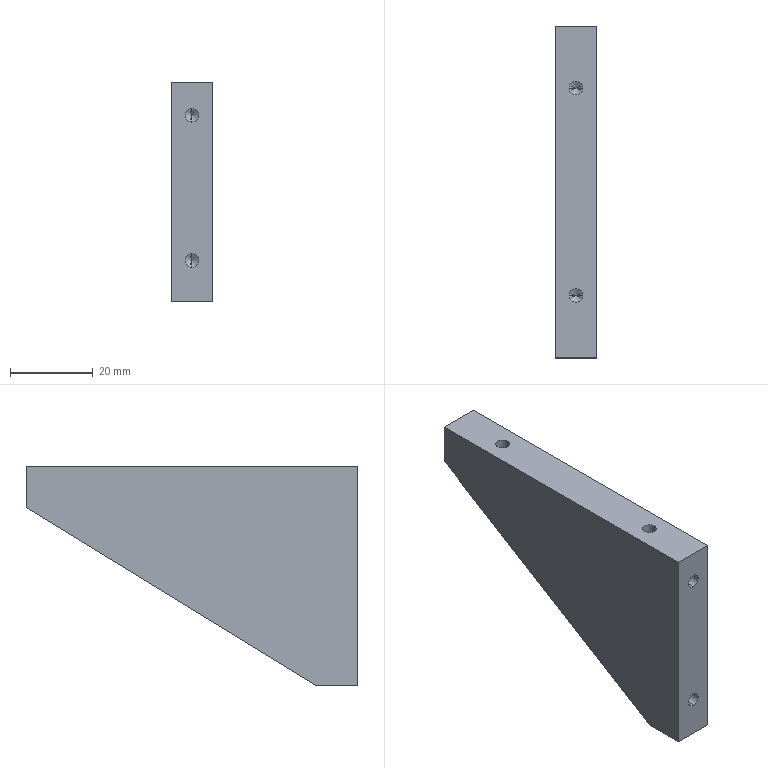Part | SolidWorks | features HoleWzd 2, Extrusion 1 | 1 solid | 23 faces | box 10 x 80 x 53 mm | volume 26993 mm3 | cylinder 8 | cone 8 | plane 7 | commonest cylinder face diameters 3.3 x8
STEP:
#1=CARTESIAN_POINT('',(5.,10.1,-41.35));
#2=VERTEX_POINT('',#1);
#3=CARTESIAN_POINT('',(5.,10.1,-44.65));
#4=VERTEX_POINT('',#3);
#5=CARTESIAN_POINT('',(5.,10.1,-43.));
#6=DIRECTION('',(0.,-1.,0.));
#7=DIRECTION('',(0.,0.,-1.));
#8=AXIS2_PLACEMENT_3D('',#5,#6,#7);
#9=CIRCLE('',#8,1.65);
#10=EDGE_CURVE('',#2,#4,#9,.T.);
#11=ORIENTED_EDGE('',*,*,#10,.F.);
#12=CARTESIAN_POINT('',(5.,0.,-41.35));
#13=VERTEX_POINT('',#12);
#14=CARTESIAN_POINT('',(5.,0.,-41.35));
#15=DIRECTION('',(0.,-1.,0.));
#16=VECTOR('',#15,1000.);
#17=LINE('',#14,#16);
#18=EDGE_CURVE('',#2,#13,#17,.T.);
#19=ORIENTED_EDGE('',*,*,#18,.T.);
#20=CARTESIAN_POINT('',(5.,0.,-44.65));
#21=VERTEX_POINT('',#20);
#22=CARTESIAN_POINT('',(5.,0.,-43.));
#23=DIRECTION('',(0.,-1.,0.));
#24=DIRECTION('',(0.,0.,-1.));
#25=AXIS2_PLACEMENT_3D('',#22,#23,#24);
#26=CIRCLE('',#25,1.65);
#27=EDGE_CURVE('',#13,#21,#26,.T.);
#28=ORIENTED_EDGE('',*,*,#27,.T.);
#29=CARTESIAN_POINT('',(5.,0.,-44.65));
#30=DIRECTION('',(0.,-1.,0.));
#31=VECTOR('',#30,1000.);
#32=LINE('',#29,#31);
#33=EDGE_CURVE('',#4,#21,#32,.T.);
#34=ORIENTED_EDGE('',*,*,#33,.F.);
#35=EDGE_LOOP('',(#11,#19,#28,#34));
#36=FACE_OUTER_BOUND('',#35,.T.);
#37=CARTESIAN_POINT('',(5.,0.,-43.));
#38=DIRECTION('',(0.,-1.,0.));
#39=DIRECTION('',(0.,0.,-1.));
#40=AXIS2_PLACEMENT_3D('',#37,#38,#39);
#41=CYLINDRICAL_SURFACE('',#40,1.65);
#42=ADVANCED_FACE('',(#36),#41,.F.);
#43=CARTESIAN_POINT('',(5.,11.091,-43.));
#44=VERTEX_POINT('',#43);
#45=CARTESIAN_POINT('',(5.,10.1,-44.65));
#46=DIRECTION('',(0.,-0.515,-0.8572));
#47=VECTOR('',#46,1000.);
#48=LINE('',#45,#47);
#49=EDGE_CURVE('',#44,#4,#48,.T.);
#50=ORIENTED_EDGE('',*,*,#49,.F.);
#51=CARTESIAN_POINT('',(5.,10.1,-41.35));
#52=DIRECTION('',(0.,-0.515,0.8572));
#53=VECTOR('',#52,1000.);
#54=LINE('',#51,#53);
#55=EDGE_CURVE('',#44,#2,#54,.T.);
#56=ORIENTED_EDGE('',*,*,#55,.T.);
#57=ORIENTED_EDGE('',*,*,#10,.T.);
#58=EDGE_LOOP('',(#50,#56,#57));
#59=FACE_OUTER_BOUND('',#58,.T.);
#60=CARTESIAN_POINT('',(5.,10.1,-43.));
#61=DIRECTION('',(0.,-1.,0.));
#62=DIRECTION('',(0.,0.,-1.));
#63=AXIS2_PLACEMENT_3D('',#60,#61,#62);
#64=CONICAL_SURFACE('',#63,1.65,1.03);
#65=ADVANCED_FACE('',(#59),#64,.F.);
#66=CARTESIAN_POINT('',(5.,10.1,-6.35));
#67=VERTEX_POINT('',#66);
#68=CARTESIAN_POINT('',(5.,10.1,-9.65));
#69=VERTEX_POINT('',#68);
#70=CARTESIAN_POINT('',(5.,10.1,-8.));
#71=DIRECTION('',(0.,-1.,0.));
#72=DIRECTION('',(0.,0.,-1.));
#73=AXIS2_PLACEMENT_3D('',#70,#71,#72);
#74=CIRCLE('',#73,1.65);
#75=EDGE_CURVE('',#67,#69,#74,.T.);
#76=ORIENTED_EDGE('',*,*,#75,.F.);
#77=CARTESIAN_POINT('',(5.,0.,-6.35));
#78=VERTEX_POINT('',#77);
#79=CARTESIAN_POINT('',(5.,0.,-6.35));
#80=DIRECTION('',(0.,-1.,0.));
#81=VECTOR('',#80,1000.);
#82=LINE('',#79,#81);
#83=EDGE_CURVE('',#67,#78,#82,.T.);
#84=ORIENTED_EDGE('',*,*,#83,.T.);
#85=CARTESIAN_POINT('',(5.,0.,-9.65));
#86=VERTEX_POINT('',#85);
#87=CARTESIAN_POINT('',(5.,0.,-8.));
#88=DIRECTION('',(0.,-1.,0.));
#89=DIRECTION('',(0.,0.,-1.));
#90=AXIS2_PLACEMENT_3D('',#87,#88,#89);
#91=CIRCLE('',#90,1.65);
#92=EDGE_CURVE('',#78,#86,#91,.T.);
#93=ORIENTED_EDGE('',*,*,#92,.T.);
#94=CARTESIAN_POINT('',(5.,0.,-9.65));
#95=DIRECTION('',(0.,-1.,0.));
#96=VECTOR('',#95,1000.);
#97=LINE('',#94,#96);
#98=EDGE_CURVE('',#69,#86,#97,.T.);
#99=ORIENTED_EDGE('',*,*,#98,.F.);
#100=EDGE_LOOP('',(#76,#84,#93,#99));
#101=FACE_OUTER_BOUND('',#100,.T.);
#102=CARTESIAN_POINT('',(5.,0.,-8.));
#103=DIRECTION('',(0.,-1.,0.));
#104=DIRECTION('',(0.,0.,-1.));
#105=AXIS2_PLACEMENT_3D('',#102,#103,#104);
#106=CYLINDRICAL_SURFACE('',#105,1.65);
#107=ADVANCED_FACE('',(#101),#106,.F.);
#108=CARTESIAN_POINT('',(5.,11.091,-8.));
#109=VERTEX_POINT('',#108);
#110=CARTESIAN_POINT('',(5.,10.1,-9.65));
#111=DIRECTION('',(0.,-0.515,-0.8572));
#112=VECTOR('',#111,1000.);
#113=LINE('',#110,#112);
#114=EDGE_CURVE('',#109,#69,#113,.T.);
#115=ORIENTED_EDGE('',*,*,#114,.F.);
#116=CARTESIAN_POINT('',(5.,10.1,-6.35));
#117=DIRECTION('',(0.,-0.515,0.8572));
#118=VECTOR('',#117,1000.);
#119=LINE('',#116,#118);
#120=EDGE_CURVE('',#109,#67,#119,.T.);
#121=ORIENTED_EDGE('',*,*,#120,.T.);
#122=ORIENTED_EDGE('',*,*,#75,.T.);
#123=EDGE_LOOP('',(#115,#121,#122));
#124=FACE_OUTER_BOUND('',#123,.T.);
#125=CARTESIAN_POINT('',(5.,10.1,-8.));
#126=DIRECTION('',(0.,-1.,0.));
#127=DIRECTION('',(0.,0.,-1.));
#128=AXIS2_PLACEMENT_3D('',#125,#126,#127);
#129=CONICAL_SURFACE('',#128,1.65,1.03);
#130=ADVANCED_FACE('',(#124),#129,.F.);
#131=CARTESIAN_POINT('',(3.35,65.,-10.1));
#132=VERTEX_POINT('',#131);
#133=CARTESIAN_POINT('',(6.65,65.,-10.1));
#134=VERTEX_POINT('',#133);
#135=CARTESIAN_POINT('',(5.,65.,-10.1));
#136=DIRECTION('',(0.,0.,1.));
#137=DIRECTION('',(1.,0.,0.));
#138=AXIS2_PLACEMENT_3D('',#135,#136,#137);
#139=CIRCLE('',#138,1.65);
#140=EDGE_CURVE('',#132,#134,#139,.T.);
#141=ORIENTED_EDGE('',*,*,#140,.F.);
#142=CARTESIAN_POINT('',(3.35,65.,0.));
#143=VERTEX_POINT('',#142);
#144=CARTESIAN_POINT('',(3.35,65.,0.));
#145=DIRECTION('',(0.,0.,1.));
#146=VECTOR('',#145,1000.);
#147=LINE('',#144,#146);
#148=EDGE_CURVE('',#132,#143,#147,.T.);
#149=ORIENTED_EDGE('',*,*,#148,.T.);
#150=CARTESIAN_POINT('',(6.65,65.,0.));
#151=VERTEX_POINT('',#150);
#152=CARTESIAN_POINT('',(5.,65.,0.));
#153=DIRECTION('',(0.,0.,1.));
#154=DIRECTION('',(1.,0.,0.));
#155=AXIS2_PLACEMENT_3D('',#152,#153,#154);
#156=CIRCLE('',#155,1.65);
#157=EDGE_CURVE('',#143,#151,#156,.T.);
#158=ORIENTED_EDGE('',*,*,#157,.T.);
#159=CARTESIAN_POINT('',(6.65,65.,0.));
#160=DIRECTION('',(0.,0.,1.));
#161=VECTOR('',#160,1000.);
#162=LINE('',#159,#161);
#163=EDGE_CURVE('',#134,#151,#162,.T.);
#164=ORIENTED_EDGE('',*,*,#163,.F.);
#165=EDGE_LOOP('',(#141,#149,#158,#164));
#166=FACE_OUTER_BOUND('',#165,.T.);
#167=CARTESIAN_POINT('',(5.,65.,0.));
#168=DIRECTION('',(0.,0.,1.));
#169=DIRECTION('',(1.,0.,0.));
#170=AXIS2_PLACEMENT_3D('',#167,#168,#169);
#171=CYLINDRICAL_SURFACE('',#170,1.65);
#172=ADVANCED_FACE('',(#166),#171,.F.);
#173=CARTESIAN_POINT('',(5.,65.,-11.091));
#174=VERTEX_POINT('',#173);
#175=CARTESIAN_POINT('',(6.65,65.,-10.1));
#176=DIRECTION('',(0.8572,0.,0.515));
#177=VECTOR('',#176,1000.);
#178=LINE('',#175,#177);
#179=EDGE_CURVE('',#174,#134,#178,.T.);
#180=ORIENTED_EDGE('',*,*,#179,.F.);
#181=CARTESIAN_POINT('',(3.35,65.,-10.1));
#182=DIRECTION('',(-0.8572,0.,0.515));
#183=VECTOR('',#182,1000.);
#184=LINE('',#181,#183);
#185=EDGE_CURVE('',#174,#132,#184,.T.);
#186=ORIENTED_EDGE('',*,*,#185,.T.);
#187=ORIENTED_EDGE('',*,*,#140,.T.);
#188=EDGE_LOOP('',(#180,#186,#187));
#189=FACE_OUTER_BOUND('',#188,.T.);
#190=CARTESIAN_POINT('',(5.,65.,-10.1));
#191=DIRECTION('',(0.,0.,1.));
#192=DIRECTION('',(1.,0.,0.));
#193=AXIS2_PLACEMENT_3D('',#190,#191,#192);
#194=CONICAL_SURFACE('',#193,1.65,1.03);
#195=ADVANCED_FACE('',(#189),#194,.F.);
#196=CARTESIAN_POINT('',(3.35,15.,-10.1));
#197=VERTEX_POINT('',#196);
#198=CARTESIAN_POINT('',(6.65,15.,-10.1));
#199=VERTEX_POINT('',#198);
#200=CARTESIAN_POINT('',(5.,15.,-10.1));
#201=DIRECTION('',(0.,0.,1.));
#202=DIRECTION('',(1.,0.,0.));
#203=AXIS2_PLACEMENT_3D('',#200,#201,#202);
#204=CIRCLE('',#203,1.65);
#205=EDGE_CURVE('',#197,#199,#204,.T.);
#206=ORIENTED_EDGE('',*,*,#205,.F.);
#207=CARTESIAN_POINT('',(3.35,15.,0.));
#208=VERTEX_POINT('',#207);
#209=CARTESIAN_POINT('',(3.35,15.,0.));
#210=DIRECTION('',(0.,0.,1.));
#211=VECTOR('',#210,1000.);
#212=LINE('',#209,#211);
#213=EDGE_CURVE('',#197,#208,#212,.T.);
#214=ORIENTED_EDGE('',*,*,#213,.T.);
#215=CARTESIAN_POINT('',(6.65,15.,0.));
#216=VERTEX_POINT('',#215);
#217=CARTESIAN_POINT('',(5.,15.,0.));
#218=DIRECTION('',(0.,0.,1.));
#219=DIRECTION('',(1.,0.,0.));
#220=AXIS2_PLACEMENT_3D('',#217,#218,#219);
#221=CIRCLE('',#220,1.65);
#222=EDGE_CURVE('',#208,#216,#221,.T.);
#223=ORIENTED_EDGE('',*,*,#222,.T.);
#224=CARTESIAN_POINT('',(6.65,15.,0.));
#225=DIRECTION('',(0.,0.,1.));
#226=VECTOR('',#225,1000.);
#227=LINE('',#224,#226);
#228=EDGE_CURVE('',#199,#216,#227,.T.);
#229=ORIENTED_EDGE('',*,*,#228,.F.);
#230=EDGE_LOOP('',(#206,#214,#223,#229));
#231=FACE_OUTER_BOUND('',#230,.T.);
#232=CARTESIAN_POINT('',(5.,15.,0.));
#233=DIRECTION('',(0.,0.,1.));
#234=DIRECTION('',(1.,0.,0.));
#235=AXIS2_PLACEMENT_3D('',#232,#233,#234);
#236=CYLINDRICAL_SURFACE('',#235,1.65);
#237=ADVANCED_FACE('',(#231),#236,.F.);
#238=CARTESIAN_POINT('',(5.,15.,-11.091));
#239=VERTEX_POINT('',#238);
#240=CARTESIAN_POINT('',(6.65,15.,-10.1));
#241=DIRECTION('',(0.8572,0.,0.515));
#242=VECTOR('',#241,1000.);
#243=LINE('',#240,#242);
#244=EDGE_CURVE('',#239,#199,#243,.T.);
#245=ORIENTED_EDGE('',*,*,#244,.F.);
#246=CARTESIAN_POINT('',(3.35,15.,-10.1));
#247=DIRECTION('',(-0.8572,0.,0.515));
#248=VECTOR('',#247,1000.);
#249=LINE('',#246,#248);
#250=EDGE_CURVE('',#239,#197,#249,.T.);
#251=ORIENTED_EDGE('',*,*,#250,.T.);
#252=ORIENTED_EDGE('',*,*,#205,.T.);
#253=EDGE_LOOP('',(#245,#251,#252));
#254=FACE_OUTER_BOUND('',#253,.T.);
#255=CARTESIAN_POINT('',(5.,15.,-10.1));
#256=DIRECTION('',(0.,0.,1.));
#257=DIRECTION('',(1.,0.,0.));
#258=AXIS2_PLACEMENT_3D('',#255,#256,#257);
#259=CONICAL_SURFACE('',#258,1.65,1.03);
#260=ADVANCED_FACE('',(#254),#259,.F.);
#261=CARTESIAN_POINT('',(5.,0.,-43.));
#262=DIRECTION('',(0.,-1.,0.));
#263=DIRECTION('',(0.,0.,-1.));
#264=AXIS2_PLACEMENT_3D('',#261,#262,#263);
#265=CIRCLE('',#264,1.65);
#266=EDGE_CURVE('',#21,#13,#265,.T.);
#267=ORIENTED_EDGE('',*,*,#266,.F.);
#268=ORIENTED_EDGE('',*,*,#27,.F.);
#269=EDGE_LOOP('',(#267,#268));
#270=FACE_BOUND('',#269,.T.);
#271=CARTESIAN_POINT('',(5.,0.,-8.));
#272=DIRECTION('',(0.,-1.,0.));
#273=DIRECTION('',(0.,0.,-1.));
#274=AXIS2_PLACEMENT_3D('',#271,#272,#273);
#275=CIRCLE('',#274,1.65);
#276=EDGE_CURVE('',#86,#78,#275,.T.);
#277=ORIENTED_EDGE('',*,*,#276,.F.);
#278=ORIENTED_EDGE('',*,*,#92,.F.);
#279=EDGE_LOOP('',(#277,#278));
#280=FACE_BOUND('',#279,.T.);
#281=CARTESIAN_POINT('',(0.,0.,0.));
#282=VERTEX_POINT('',#281);
#283=CARTESIAN_POINT('',(0.,0.,-53.));
#284=VERTEX_POINT('',#283);
#285=CARTESIAN_POINT('',(0.,0.,-53.));
#286=DIRECTION('',(0.,0.,-1.));
#287=VECTOR('',#286,1000.);
#288=LINE('',#285,#287);
#289=EDGE_CURVE('',#282,#284,#288,.T.);
#290=ORIENTED_EDGE('',*,*,#289,.T.);
#291=CARTESIAN_POINT('',(10.,0.,-53.));
#292=VERTEX_POINT('',#291);
#293=CARTESIAN_POINT('',(10.,0.,-53.));
#294=DIRECTION('',(-1.,0.,0.));
#295=VECTOR('',#294,1000.);
#296=LINE('',#293,#295);
#297=EDGE_CURVE('',#292,#284,#296,.T.);
#298=ORIENTED_EDGE('',*,*,#297,.F.);
#299=CARTESIAN_POINT('',(10.,0.,0.));
#300=VERTEX_POINT('',#299);
#301=CARTESIAN_POINT('',(10.,0.,-53.));
#302=DIRECTION('',(0.,0.,-1.));
#303=VECTOR('',#302,1000.);
#304=LINE('',#301,#303);
#305=EDGE_CURVE('',#300,#292,#304,.T.);
#306=ORIENTED_EDGE('',*,*,#305,.F.);
#307=CARTESIAN_POINT('',(10.,0.,0.));
#308=DIRECTION('',(-1.,0.,0.));
#309=VECTOR('',#308,1000.);
#310=LINE('',#307,#309);
#311=EDGE_CURVE('',#300,#282,#310,.T.);
#312=ORIENTED_EDGE('',*,*,#311,.T.);
#313=EDGE_LOOP('',(#290,#298,#306,#312));
#314=FACE_OUTER_BOUND('',#313,.T.);
#315=CARTESIAN_POINT('',(10.,0.,-53.));
#316=DIRECTION('',(0.,1.,0.));
#317=DIRECTION('',(0.,0.,1.));
#318=AXIS2_PLACEMENT_3D('',#315,#316,#317);
#319=PLANE('',#318);
#320=ADVANCED_FACE('',(#270,#280,#314),#319,.F.);
#321=CARTESIAN_POINT('',(0.,10.,-53.));
#322=VERTEX_POINT('',#321);
#323=CARTESIAN_POINT('',(0.,10.,-53.));
#324=DIRECTION('',(0.,1.,0.));
#325=VECTOR('',#324,1000.);
#326=LINE('',#323,#325);
#327=EDGE_CURVE('',#284,#322,#326,.T.);
#328=ORIENTED_EDGE('',*,*,#327,.T.);
#329=CARTESIAN_POINT('',(10.,10.,-53.));
#330=VERTEX_POINT('',#329);
#331=CARTESIAN_POINT('',(10.,10.,-53.));
#332=DIRECTION('',(-1.,0.,0.));
#333=VECTOR('',#332,1000.);
#334=LINE('',#331,#333);
#335=EDGE_CURVE('',#330,#322,#334,.T.);
#336=ORIENTED_EDGE('',*,*,#335,.F.);
#337=CARTESIAN_POINT('',(10.,10.,-53.));
#338=DIRECTION('',(0.,1.,0.));
#339=VECTOR('',#338,1000.);
#340=LINE('',#337,#339);
#341=EDGE_CURVE('',#292,#330,#340,.T.);
#342=ORIENTED_EDGE('',*,*,#341,.F.);
#343=ORIENTED_EDGE('',*,*,#297,.T.);
#344=EDGE_LOOP('',(#328,#336,#342,#343));
#345=FACE_OUTER_BOUND('',#344,.T.);
#346=CARTESIAN_POINT('',(10.,10.,-53.));
#347=DIRECTION('',(0.,0.,1.));
#348=DIRECTION('',(1.,0.,0.));
#349=AXIS2_PLACEMENT_3D('',#346,#347,#348);
#350=PLANE('',#349);
#351=ADVANCED_FACE('',(#345),#350,.F.);
#352=CARTESIAN_POINT('',(0.,80.,-10.));
#353=VERTEX_POINT('',#352);
#354=CARTESIAN_POINT('',(0.,80.,-10.));
#355=DIRECTION('',(0.,0.8521,0.5234));
#356=VECTOR('',#355,1000.);
#357=LINE('',#354,#356);
#358=EDGE_CURVE('',#322,#353,#357,.T.);
#359=ORIENTED_EDGE('',*,*,#358,.T.);
#360=CARTESIAN_POINT('',(10.,80.,-10.));
#361=VERTEX_POINT('',#360);
#362=CARTESIAN_POINT('',(10.,80.,-10.));
#363=DIRECTION('',(-1.,0.,0.));
#364=VECTOR('',#363,1000.);
#365=LINE('',#362,#364);
#366=EDGE_CURVE('',#361,#353,#365,.T.);
#367=ORIENTED_EDGE('',*,*,#366,.F.);
#368=CARTESIAN_POINT('',(10.,80.,-10.));
#369=DIRECTION('',(0.,0.8521,0.5234));
#370=VECTOR('',#369,1000.);
#371=LINE('',#368,#370);
#372=EDGE_CURVE('',#330,#361,#371,.T.);
#373=ORIENTED_EDGE('',*,*,#372,.F.);
#374=ORIENTED_EDGE('',*,*,#335,.T.);
#375=EDGE_LOOP('',(#359,#367,#373,#374));
#376=FACE_OUTER_BOUND('',#375,.T.);
#377=CARTESIAN_POINT('',(10.,80.,-10.));
#378=DIRECTION('',(0.,-0.5234,0.8521));
#379=DIRECTION('',(0.,-0.8521,-0.5234));
#380=AXIS2_PLACEMENT_3D('',#377,#378,#379);
#381=PLANE('',#380);
#382=ADVANCED_FACE('',(#376),#381,.F.);
#383=CARTESIAN_POINT('',(0.,80.,0.));
#384=VERTEX_POINT('',#383);
#385=CARTESIAN_POINT('',(0.,80.,0.));
#386=DIRECTION('',(0.,0.,1.));
#387=VECTOR('',#386,1000.);
#388=LINE('',#385,#387);
#389=EDGE_CURVE('',#353,#384,#388,.T.);
#390=ORIENTED_EDGE('',*,*,#389,.T.);
#391=CARTESIAN_POINT('',(10.,80.,0.));
#392=VERTEX_POINT('',#391);
#393=CARTESIAN_POINT('',(10.,80.,0.));
#394=DIRECTION('',(-1.,0.,0.));
#395=VECTOR('',#394,1000.);
#396=LINE('',#393,#395);
#397=EDGE_CURVE('',#392,#384,#396,.T.);
#398=ORIENTED_EDGE('',*,*,#397,.F.);
#399=CARTESIAN_POINT('',(10.,80.,0.));
#400=DIRECTION('',(0.,0.,1.));
#401=VECTOR('',#400,1000.);
#402=LINE('',#399,#401);
#403=EDGE_CURVE('',#361,#392,#402,.T.);
#404=ORIENTED_EDGE('',*,*,#403,.F.);
#405=ORIENTED_EDGE('',*,*,#366,.T.);
#406=EDGE_LOOP('',(#390,#398,#404,#405));
#407=FACE_OUTER_BOUND('',#406,.T.);
#408=CARTESIAN_POINT('',(10.,80.,0.));
#409=DIRECTION('',(0.,-1.,0.));
#410=DIRECTION('',(0.,0.,-1.));
#411=AXIS2_PLACEMENT_3D('',#408,#409,#410);
#412=PLANE('',#411);
#413=ADVANCED_FACE('',(#407),#412,.F.);
#414=CARTESIAN_POINT('',(5.,65.,0.));
#415=DIRECTION('',(0.,0.,1.));
#416=DIRECTION('',(1.,0.,0.));
#417=AXIS2_PLACEMENT_3D('',#414,#415,#416);
#418=CIRCLE('',#417,1.65);
#419=EDGE_CURVE('',#151,#143,#418,.T.);
#420=ORIENTED_EDGE('',*,*,#419,.F.);
#421=ORIENTED_EDGE('',*,*,#157,.F.);
#422=EDGE_LOOP('',(#420,#421));
#423=FACE_BOUND('',#422,.T.);
#424=CARTESIAN_POINT('',(5.,15.,0.));
#425=DIRECTION('',(0.,0.,1.));
#426=DIRECTION('',(1.,0.,0.));
#427=AXIS2_PLACEMENT_3D('',#424,#425,#426);
#428=CIRCLE('',#427,1.65);
#429=EDGE_CURVE('',#216,#208,#428,.T.);
#430=ORIENTED_EDGE('',*,*,#429,.F.);
#431=ORIENTED_EDGE('',*,*,#222,.F.);
#432=EDGE_LOOP('',(#430,#431));
#433=FACE_BOUND('',#432,.T.);
#434=CARTESIAN_POINT('',(0.,0.,0.));
#435=DIRECTION('',(0.,-1.,0.));
#436=VECTOR('',#435,1000.);
#437=LINE('',#434,#436);
#438=EDGE_CURVE('',#384,#282,#437,.T.);
#439=ORIENTED_EDGE('',*,*,#438,.T.);
#440=ORIENTED_EDGE('',*,*,#311,.F.);
#441=CARTESIAN_POINT('',(10.,0.,0.));
#442=DIRECTION('',(0.,-1.,0.));
#443=VECTOR('',#442,1000.);
#444=LINE('',#441,#443);
#445=EDGE_CURVE('',#392,#300,#444,.T.);
#446=ORIENTED_EDGE('',*,*,#445,.F.);
#447=ORIENTED_EDGE('',*,*,#397,.T.);
#448=EDGE_LOOP('',(#439,#440,#446,#447));
#449=FACE_OUTER_BOUND('',#448,.T.);
#450=CARTESIAN_POINT('',(10.,0.,0.));
#451=DIRECTION('',(0.,0.,-1.));
#452=DIRECTION('',(-1.,0.,0.));
#453=AXIS2_PLACEMENT_3D('',#450,#451,#452);
#454=PLANE('',#453);
#455=ADVANCED_FACE('',(#423,#433,#449),#454,.F.);
#456=ORIENTED_EDGE('',*,*,#305,.T.);
#457=ORIENTED_EDGE('',*,*,#341,.T.);
#458=ORIENTED_EDGE('',*,*,#372,.T.);
#459=ORIENTED_EDGE('',*,*,#403,.T.);
#460=ORIENTED_EDGE('',*,*,#445,.T.);
#461=EDGE_LOOP('',(#456,#457,#458,#459,#460));
#462=FACE_OUTER_BOUND('',#461,.T.);
#463=CARTESIAN_POINT('',(10.,0.,0.));
#464=DIRECTION('',(-1.,0.,0.));
#465=DIRECTION('',(0.,0.,1.));
#466=AXIS2_PLACEMENT_3D('',#463,#464,#465);
#467=PLANE('',#466);
#468=ADVANCED_FACE('',(#462),#467,.F.);
#469=ORIENTED_EDGE('',*,*,#289,.F.);
#470=ORIENTED_EDGE('',*,*,#438,.F.);
#471=ORIENTED_EDGE('',*,*,#389,.F.);
#472=ORIENTED_EDGE('',*,*,#358,.F.);
#473=ORIENTED_EDGE('',*,*,#327,.F.);
#474=EDGE_LOOP('',(#469,#470,#471,#472,#473));
#475=FACE_OUTER_BOUND('',#474,.T.);
#476=CARTESIAN_POINT('',(0.,0.,0.));
#477=DIRECTION('',(-1.,0.,0.));
#478=DIRECTION('',(0.,0.,1.));
#479=AXIS2_PLACEMENT_3D('',#476,#477,#478);
#480=PLANE('',#479);
#481=ADVANCED_FACE('',(#475),#480,.T.);
#482=ORIENTED_EDGE('',*,*,#250,.F.);
#483=ORIENTED_EDGE('',*,*,#244,.T.);
#484=CARTESIAN_POINT('',(5.,15.,-10.1));
#485=DIRECTION('',(0.,0.,1.));
#486=DIRECTION('',(1.,0.,0.));
#487=AXIS2_PLACEMENT_3D('',#484,#485,#486);
#488=CIRCLE('',#487,1.65);
#489=EDGE_CURVE('',#199,#197,#488,.T.);
#490=ORIENTED_EDGE('',*,*,#489,.T.);
#491=EDGE_LOOP('',(#482,#483,#490));
#492=FACE_OUTER_BOUND('',#491,.T.);
#493=CARTESIAN_POINT('',(5.,15.,-10.1));
#494=DIRECTION('',(0.,0.,1.));
#495=DIRECTION('',(1.,0.,0.));
#496=AXIS2_PLACEMENT_3D('',#493,#494,#495);
#497=CONICAL_SURFACE('',#496,1.65,1.03);
#498=ADVANCED_FACE('',(#492),#497,.F.);
#499=ORIENTED_EDGE('',*,*,#213,.F.);
#500=ORIENTED_EDGE('',*,*,#489,.F.);
#501=ORIENTED_EDGE('',*,*,#228,.T.);
#502=ORIENTED_EDGE('',*,*,#429,.T.);
#503=EDGE_LOOP('',(#499,#500,#501,#502));
#504=FACE_OUTER_BOUND('',#503,.T.);
#505=CARTESIAN_POINT('',(5.,15.,0.));
#506=DIRECTION('',(0.,0.,1.));
#507=DIRECTION('',(1.,0.,0.));
#508=AXIS2_PLACEMENT_3D('',#505,#506,#507);
#509=CYLINDRICAL_SURFACE('',#508,1.65);
#510=ADVANCED_FACE('',(#504),#509,.F.);
#511=ORIENTED_EDGE('',*,*,#185,.F.);
#512=ORIENTED_EDGE('',*,*,#179,.T.);
#513=CARTESIAN_POINT('',(5.,65.,-10.1));
#514=DIRECTION('',(0.,0.,1.));
#515=DIRECTION('',(1.,0.,0.));
#516=AXIS2_PLACEMENT_3D('',#513,#514,#515);
#517=CIRCLE('',#516,1.65);
#518=EDGE_CURVE('',#134,#132,#517,.T.);
#519=ORIENTED_EDGE('',*,*,#518,.T.);
#520=EDGE_LOOP('',(#511,#512,#519));
#521=FACE_OUTER_BOUND('',#520,.T.);
#522=CARTESIAN_POINT('',(5.,65.,-10.1));
#523=DIRECTION('',(0.,0.,1.));
#524=DIRECTION('',(1.,0.,0.));
#525=AXIS2_PLACEMENT_3D('',#522,#523,#524);
#526=CONICAL_SURFACE('',#525,1.65,1.03);
#527=ADVANCED_FACE('',(#521),#526,.F.);
#528=ORIENTED_EDGE('',*,*,#148,.F.);
#529=ORIENTED_EDGE('',*,*,#518,.F.);
#530=ORIENTED_EDGE('',*,*,#163,.T.);
#531=ORIENTED_EDGE('',*,*,#419,.T.);
#532=EDGE_LOOP('',(#528,#529,#530,#531));
#533=FACE_OUTER_BOUND('',#532,.T.);
#534=CARTESIAN_POINT('',(5.,65.,0.));
#535=DIRECTION('',(0.,0.,1.));
#536=DIRECTION('',(1.,0.,0.));
#537=AXIS2_PLACEMENT_3D('',#534,#535,#536);
#538=CYLINDRICAL_SURFACE('',#537,1.65);
#539=ADVANCED_FACE('',(#533),#538,.F.);
#540=ORIENTED_EDGE('',*,*,#120,.F.);
#541=ORIENTED_EDGE('',*,*,#114,.T.);
#542=CARTESIAN_POINT('',(5.,10.1,-8.));
#543=DIRECTION('',(0.,-1.,0.));
#544=DIRECTION('',(0.,0.,-1.));
#545=AXIS2_PLACEMENT_3D('',#542,#543,#544);
#546=CIRCLE('',#545,1.65);
#547=EDGE_CURVE('',#69,#67,#546,.T.);
#548=ORIENTED_EDGE('',*,*,#547,.T.);
#549=EDGE_LOOP('',(#540,#541,#548));
#550=FACE_OUTER_BOUND('',#549,.T.);
#551=CARTESIAN_POINT('',(5.,10.1,-8.));
#552=DIRECTION('',(0.,-1.,0.));
#553=DIRECTION('',(0.,0.,-1.));
#554=AXIS2_PLACEMENT_3D('',#551,#552,#553);
#555=CONICAL_SURFACE('',#554,1.65,1.03);
#556=ADVANCED_FACE('',(#550),#555,.F.);
#557=ORIENTED_EDGE('',*,*,#83,.F.);
#558=ORIENTED_EDGE('',*,*,#547,.F.);
#559=ORIENTED_EDGE('',*,*,#98,.T.);
#560=ORIENTED_EDGE('',*,*,#276,.T.);
#561=EDGE_LOOP('',(#557,#558,#559,#560));
#562=FACE_OUTER_BOUND('',#561,.T.);
#563=CARTESIAN_POINT('',(5.,0.,-8.));
#564=DIRECTION('',(0.,-1.,0.));
#565=DIRECTION('',(0.,0.,-1.));
#566=AXIS2_PLACEMENT_3D('',#563,#564,#565);
#567=CYLINDRICAL_SURFACE('',#566,1.65);
#568=ADVANCED_FACE('',(#562),#567,.F.);
#569=ORIENTED_EDGE('',*,*,#55,.F.);
#570=ORIENTED_EDGE('',*,*,#49,.T.);
#571=CARTESIAN_POINT('',(5.,10.1,-43.));
#572=DIRECTION('',(0.,-1.,0.));
#573=DIRECTION('',(0.,0.,-1.));
#574=AXIS2_PLACEMENT_3D('',#571,#572,#573);
#575=CIRCLE('',#574,1.65);
#576=EDGE_CURVE('',#4,#2,#575,.T.);
#577=ORIENTED_EDGE('',*,*,#576,.T.);
#578=EDGE_LOOP('',(#569,#570,#577));
#579=FACE_OUTER_BOUND('',#578,.T.);
#580=CARTESIAN_POINT('',(5.,10.1,-43.));
#581=DIRECTION('',(0.,-1.,0.));
#582=DIRECTION('',(0.,0.,-1.));
#583=AXIS2_PLACEMENT_3D('',#580,#581,#582);
#584=CONICAL_SURFACE('',#583,1.65,1.03);
#585=ADVANCED_FACE('',(#579),#584,.F.);
#586=ORIENTED_EDGE('',*,*,#18,.F.);
#587=ORIENTED_EDGE('',*,*,#576,.F.);
#588=ORIENTED_EDGE('',*,*,#33,.T.);
#589=ORIENTED_EDGE('',*,*,#266,.T.);
#590=EDGE_LOOP('',(#586,#587,#588,#589));
#591=FACE_OUTER_BOUND('',#590,.T.);
#592=CARTESIAN_POINT('',(5.,0.,-43.));
#593=DIRECTION('',(0.,-1.,0.));
#594=DIRECTION('',(0.,0.,-1.));
#595=AXIS2_PLACEMENT_3D('',#592,#593,#594);
#596=CYLINDRICAL_SURFACE('',#595,1.65);
#597=ADVANCED_FACE('',(#591),#596,.F.);
#598=CLOSED_SHELL('',(#42,#65,#107,#130,#172,#195,#237,#260,#320,#351,#382,#413,#455,#468,#481,#498,#510,#527,#539,#556,#568,#585,#597));
#599=MANIFOLD_SOLID_BREP('',#598);
#600=CARTESIAN_POINT('',(0.,0.,0.));
#601=DIRECTION('',(0.,0.,1.));
#602=DIRECTION('',(1.,0.,0.));
#603=AXIS2_PLACEMENT_3D('',#600,#601,#602);
#604=(LENGTH_UNIT()NAMED_UNIT(*)SI_UNIT(.MILLI.,.METRE.));
#605=UNCERTAINTY_MEASURE_WITH_UNIT(LENGTH_MEASURE(0.00001),#604,'','');
#606=(NAMED_UNIT(*)PLANE_ANGLE_UNIT()SI_UNIT($,.RADIAN.));
#607=(NAMED_UNIT(*)SI_UNIT($,.STERADIAN.)SOLID_ANGLE_UNIT());
#608=(GEOMETRIC_REPRESENTATION_CONTEXT(3)GLOBAL_UNCERTAINTY_ASSIGNED_CONTEXT((#605))GLOBAL_UNIT_ASSIGNED_CONTEXT((#604,#606,#607))REPRESENTATION_CONTEXT('',''));
#609=ADVANCED_BREP_SHAPE_REPRESENTATION('',(#599,#603),#608);